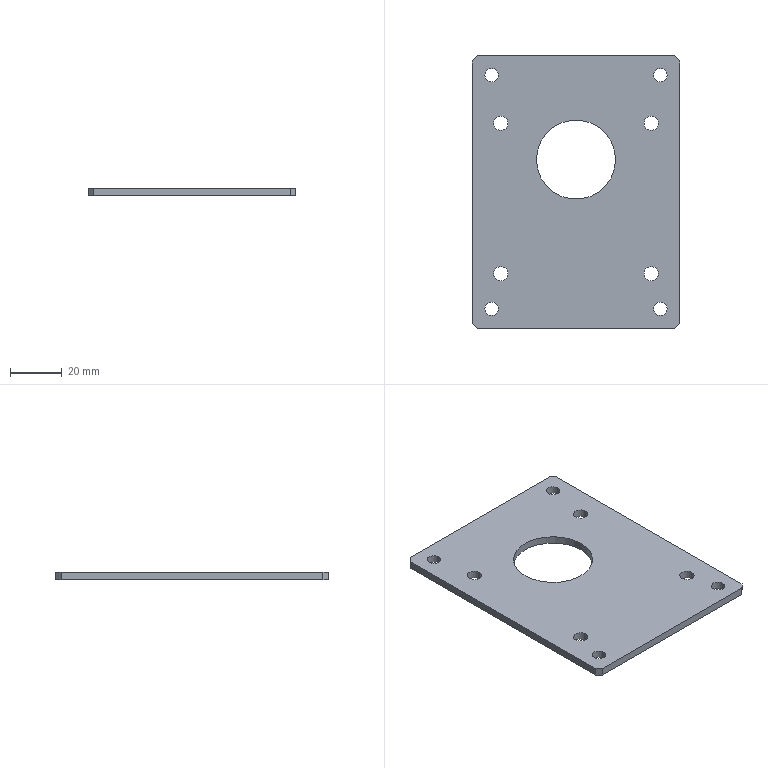Part | SolidWorks | features ICE 2, Chamfer 1, Extrusion 1, HoleWzd 1 | 1 solid | 28 faces | box 80 x 105 x 3 mm | volume 22444 mm3 | cylinder 18 | plane 10 | commonest cylinder face diameters 5.2 x8 5.5 x8 30.5 x2
STEP:
#1=CARTESIAN_POINT('',(13.759,21.009,3.));
#2=VERTEX_POINT('',#1);
#3=CARTESIAN_POINT('',(8.259,21.009,3.));
#4=VERTEX_POINT('',#3);
#5=CARTESIAN_POINT('',(11.009,21.009,3.));
#6=DIRECTION('',(0.,0.,-1.));
#7=DIRECTION('',(-1.,0.,0.));
#8=AXIS2_PLACEMENT_3D('',#5,#6,#7);
#9=CIRCLE('',#8,2.75);
#10=EDGE_CURVE('',#2,#4,#9,.T.);
#11=ORIENTED_EDGE('',*,*,#10,.F.);
#12=CARTESIAN_POINT('',(13.759,21.009,0.));
#13=VERTEX_POINT('',#12);
#14=CARTESIAN_POINT('',(13.759,21.009,3.));
#15=DIRECTION('',(0.,0.,-1.));
#16=VECTOR('',#15,1000.);
#17=LINE('',#14,#16);
#18=EDGE_CURVE('',#2,#13,#17,.T.);
#19=ORIENTED_EDGE('',*,*,#18,.T.);
#20=CARTESIAN_POINT('',(8.259,21.009,0.));
#21=VERTEX_POINT('',#20);
#22=CARTESIAN_POINT('',(11.009,21.009,0.));
#23=DIRECTION('',(0.,0.,-1.));
#24=DIRECTION('',(-1.,0.,0.));
#25=AXIS2_PLACEMENT_3D('',#22,#23,#24);
#26=CIRCLE('',#25,2.75);
#27=EDGE_CURVE('',#13,#21,#26,.T.);
#28=ORIENTED_EDGE('',*,*,#27,.T.);
#29=CARTESIAN_POINT('',(8.259,21.009,3.));
#30=DIRECTION('',(0.,0.,-1.));
#31=VECTOR('',#30,1000.);
#32=LINE('',#29,#31);
#33=EDGE_CURVE('',#4,#21,#32,.T.);
#34=ORIENTED_EDGE('',*,*,#33,.F.);
#35=EDGE_LOOP('',(#11,#19,#28,#34));
#36=FACE_OUTER_BOUND('',#35,.T.);
#37=CARTESIAN_POINT('',(11.009,21.009,3.));
#38=DIRECTION('',(0.,0.,-1.));
#39=DIRECTION('',(-1.,0.,0.));
#40=AXIS2_PLACEMENT_3D('',#37,#38,#39);
#41=CYLINDRICAL_SURFACE('',#40,2.75);
#42=ADVANCED_FACE('',(#36),#41,.F.);
#43=CARTESIAN_POINT('',(71.741,21.009,3.));
#44=VERTEX_POINT('',#43);
#45=CARTESIAN_POINT('',(66.241,21.009,3.));
#46=VERTEX_POINT('',#45);
#47=CARTESIAN_POINT('',(68.991,21.009,3.));
#48=DIRECTION('',(0.,0.,-1.));
#49=DIRECTION('',(-1.,0.,0.));
#50=AXIS2_PLACEMENT_3D('',#47,#48,#49);
#51=CIRCLE('',#50,2.75);
#52=EDGE_CURVE('',#44,#46,#51,.T.);
#53=ORIENTED_EDGE('',*,*,#52,.F.);
#54=CARTESIAN_POINT('',(71.741,21.009,0.));
#55=VERTEX_POINT('',#54);
#56=CARTESIAN_POINT('',(71.741,21.009,3.));
#57=DIRECTION('',(0.,0.,-1.));
#58=VECTOR('',#57,1000.);
#59=LINE('',#56,#58);
#60=EDGE_CURVE('',#44,#55,#59,.T.);
#61=ORIENTED_EDGE('',*,*,#60,.T.);
#62=CARTESIAN_POINT('',(66.241,21.009,0.));
#63=VERTEX_POINT('',#62);
#64=CARTESIAN_POINT('',(68.991,21.009,0.));
#65=DIRECTION('',(0.,0.,-1.));
#66=DIRECTION('',(-1.,0.,0.));
#67=AXIS2_PLACEMENT_3D('',#64,#65,#66);
#68=CIRCLE('',#67,2.75);
#69=EDGE_CURVE('',#55,#63,#68,.T.);
#70=ORIENTED_EDGE('',*,*,#69,.T.);
#71=CARTESIAN_POINT('',(66.241,21.009,3.));
#72=DIRECTION('',(0.,0.,-1.));
#73=VECTOR('',#72,1000.);
#74=LINE('',#71,#73);
#75=EDGE_CURVE('',#46,#63,#74,.T.);
#76=ORIENTED_EDGE('',*,*,#75,.F.);
#77=EDGE_LOOP('',(#53,#61,#70,#76));
#78=FACE_OUTER_BOUND('',#77,.T.);
#79=CARTESIAN_POINT('',(68.991,21.009,3.));
#80=DIRECTION('',(0.,0.,-1.));
#81=DIRECTION('',(-1.,0.,0.));
#82=AXIS2_PLACEMENT_3D('',#79,#80,#81);
#83=CYLINDRICAL_SURFACE('',#82,2.75);
#84=ADVANCED_FACE('',(#78),#83,.F.);
#85=CARTESIAN_POINT('',(13.759,78.991,3.));
#86=VERTEX_POINT('',#85);
#87=CARTESIAN_POINT('',(8.259,78.991,3.));
#88=VERTEX_POINT('',#87);
#89=CARTESIAN_POINT('',(11.009,78.991,3.));
#90=DIRECTION('',(0.,0.,-1.));
#91=DIRECTION('',(-1.,0.,0.));
#92=AXIS2_PLACEMENT_3D('',#89,#90,#91);
#93=CIRCLE('',#92,2.75);
#94=EDGE_CURVE('',#86,#88,#93,.T.);
#95=ORIENTED_EDGE('',*,*,#94,.F.);
#96=CARTESIAN_POINT('',(13.759,78.991,0.));
#97=VERTEX_POINT('',#96);
#98=CARTESIAN_POINT('',(13.759,78.991,3.));
#99=DIRECTION('',(0.,0.,-1.));
#100=VECTOR('',#99,1000.);
#101=LINE('',#98,#100);
#102=EDGE_CURVE('',#86,#97,#101,.T.);
#103=ORIENTED_EDGE('',*,*,#102,.T.);
#104=CARTESIAN_POINT('',(8.259,78.991,0.));
#105=VERTEX_POINT('',#104);
#106=CARTESIAN_POINT('',(11.009,78.991,0.));
#107=DIRECTION('',(0.,0.,-1.));
#108=DIRECTION('',(-1.,0.,0.));
#109=AXIS2_PLACEMENT_3D('',#106,#107,#108);
#110=CIRCLE('',#109,2.75);
#111=EDGE_CURVE('',#97,#105,#110,.T.);
#112=ORIENTED_EDGE('',*,*,#111,.T.);
#113=CARTESIAN_POINT('',(8.259,78.991,3.));
#114=DIRECTION('',(0.,0.,-1.));
#115=VECTOR('',#114,1000.);
#116=LINE('',#113,#115);
#117=EDGE_CURVE('',#88,#105,#116,.T.);
#118=ORIENTED_EDGE('',*,*,#117,.F.);
#119=EDGE_LOOP('',(#95,#103,#112,#118));
#120=FACE_OUTER_BOUND('',#119,.T.);
#121=CARTESIAN_POINT('',(11.009,78.991,3.));
#122=DIRECTION('',(0.,0.,-1.));
#123=DIRECTION('',(-1.,0.,0.));
#124=AXIS2_PLACEMENT_3D('',#121,#122,#123);
#125=CYLINDRICAL_SURFACE('',#124,2.75);
#126=ADVANCED_FACE('',(#120),#125,.F.);
#127=CARTESIAN_POINT('',(71.741,78.991,3.));
#128=VERTEX_POINT('',#127);
#129=CARTESIAN_POINT('',(66.241,78.991,3.));
#130=VERTEX_POINT('',#129);
#131=CARTESIAN_POINT('',(68.991,78.991,3.));
#132=DIRECTION('',(0.,0.,-1.));
#133=DIRECTION('',(-1.,0.,0.));
#134=AXIS2_PLACEMENT_3D('',#131,#132,#133);
#135=CIRCLE('',#134,2.75);
#136=EDGE_CURVE('',#128,#130,#135,.T.);
#137=ORIENTED_EDGE('',*,*,#136,.F.);
#138=CARTESIAN_POINT('',(71.741,78.991,0.));
#139=VERTEX_POINT('',#138);
#140=CARTESIAN_POINT('',(71.741,78.991,3.));
#141=DIRECTION('',(0.,0.,-1.));
#142=VECTOR('',#141,1000.);
#143=LINE('',#140,#142);
#144=EDGE_CURVE('',#128,#139,#143,.T.);
#145=ORIENTED_EDGE('',*,*,#144,.T.);
#146=CARTESIAN_POINT('',(66.241,78.991,0.));
#147=VERTEX_POINT('',#146);
#148=CARTESIAN_POINT('',(68.991,78.991,0.));
#149=DIRECTION('',(0.,0.,-1.));
#150=DIRECTION('',(-1.,0.,0.));
#151=AXIS2_PLACEMENT_3D('',#148,#149,#150);
#152=CIRCLE('',#151,2.75);
#153=EDGE_CURVE('',#139,#147,#152,.T.);
#154=ORIENTED_EDGE('',*,*,#153,.T.);
#155=CARTESIAN_POINT('',(66.241,78.991,3.));
#156=DIRECTION('',(0.,0.,-1.));
#157=VECTOR('',#156,1000.);
#158=LINE('',#155,#157);
#159=EDGE_CURVE('',#130,#147,#158,.T.);
#160=ORIENTED_EDGE('',*,*,#159,.F.);
#161=EDGE_LOOP('',(#137,#145,#154,#160));
#162=FACE_OUTER_BOUND('',#161,.T.);
#163=CARTESIAN_POINT('',(68.991,78.991,3.));
#164=DIRECTION('',(0.,0.,-1.));
#165=DIRECTION('',(-1.,0.,0.));
#166=AXIS2_PLACEMENT_3D('',#163,#164,#165);
#167=CYLINDRICAL_SURFACE('',#166,2.75);
#168=ADVANCED_FACE('',(#162),#167,.F.);
#169=CARTESIAN_POINT('',(55.25,65.,0.));
#170=VERTEX_POINT('',#169);
#171=CARTESIAN_POINT('',(24.75,65.,0.));
#172=VERTEX_POINT('',#171);
#173=CARTESIAN_POINT('',(40.,65.,0.));
#174=DIRECTION('',(0.,0.,-1.));
#175=DIRECTION('',(-1.,0.,0.));
#176=AXIS2_PLACEMENT_3D('',#173,#174,#175);
#177=CIRCLE('',#176,15.25);
#178=EDGE_CURVE('',#170,#172,#177,.T.);
#179=ORIENTED_EDGE('',*,*,#178,.T.);
#180=CARTESIAN_POINT('',(24.75,65.,3.));
#181=VERTEX_POINT('',#180);
#182=CARTESIAN_POINT('',(24.75,65.,-7.));
#183=DIRECTION('',(0.,0.,1.));
#184=VECTOR('',#183,1000.);
#185=LINE('',#182,#184);
#186=EDGE_CURVE('',#172,#181,#185,.T.);
#187=ORIENTED_EDGE('',*,*,#186,.T.);
#188=CARTESIAN_POINT('',(55.25,65.,3.));
#189=VERTEX_POINT('',#188);
#190=CARTESIAN_POINT('',(40.,65.,3.));
#191=DIRECTION('',(0.,0.,1.));
#192=DIRECTION('',(1.,0.,0.));
#193=AXIS2_PLACEMENT_3D('',#190,#191,#192);
#194=CIRCLE('',#193,15.25);
#195=EDGE_CURVE('',#181,#189,#194,.T.);
#196=ORIENTED_EDGE('',*,*,#195,.T.);
#197=CARTESIAN_POINT('',(55.25,65.,-7.));
#198=DIRECTION('',(0.,0.,1.));
#199=VECTOR('',#198,1000.);
#200=LINE('',#197,#199);
#201=EDGE_CURVE('',#170,#189,#200,.T.);
#202=ORIENTED_EDGE('',*,*,#201,.F.);
#203=EDGE_LOOP('',(#179,#187,#196,#202));
#204=FACE_OUTER_BOUND('',#203,.T.);
#205=CARTESIAN_POINT('',(40.,65.,-7.));
#206=DIRECTION('',(0.,0.,1.));
#207=DIRECTION('',(1.,0.,0.));
#208=AXIS2_PLACEMENT_3D('',#205,#206,#207);
#209=CYLINDRICAL_SURFACE('',#208,15.25);
#210=ADVANCED_FACE('',(#204),#209,.F.);
#211=CARTESIAN_POINT('',(75.1,7.5,0.));
#212=VERTEX_POINT('',#211);
#213=CARTESIAN_POINT('',(69.9,7.5,0.));
#214=VERTEX_POINT('',#213);
#215=CARTESIAN_POINT('',(72.5,7.5,0.));
#216=DIRECTION('',(0.,0.,-1.));
#217=DIRECTION('',(-1.,0.,0.));
#218=AXIS2_PLACEMENT_3D('',#215,#216,#217);
#219=CIRCLE('',#218,2.6);
#220=EDGE_CURVE('',#212,#214,#219,.T.);
#221=ORIENTED_EDGE('',*,*,#220,.T.);
#222=CARTESIAN_POINT('',(69.9,7.5,3.));
#223=VERTEX_POINT('',#222);
#224=CARTESIAN_POINT('',(69.9,7.5,-7.));
#225=DIRECTION('',(0.,0.,1.));
#226=VECTOR('',#225,1000.);
#227=LINE('',#224,#226);
#228=EDGE_CURVE('',#214,#223,#227,.T.);
#229=ORIENTED_EDGE('',*,*,#228,.T.);
#230=CARTESIAN_POINT('',(75.1,7.5,3.));
#231=VERTEX_POINT('',#230);
#232=CARTESIAN_POINT('',(72.5,7.5,3.));
#233=DIRECTION('',(0.,0.,1.));
#234=DIRECTION('',(1.,0.,0.));
#235=AXIS2_PLACEMENT_3D('',#232,#233,#234);
#236=CIRCLE('',#235,2.6);
#237=EDGE_CURVE('',#223,#231,#236,.T.);
#238=ORIENTED_EDGE('',*,*,#237,.T.);
#239=CARTESIAN_POINT('',(75.1,7.5,-7.));
#240=DIRECTION('',(0.,0.,1.));
#241=VECTOR('',#240,1000.);
#242=LINE('',#239,#241);
#243=EDGE_CURVE('',#212,#231,#242,.T.);
#244=ORIENTED_EDGE('',*,*,#243,.F.);
#245=EDGE_LOOP('',(#221,#229,#238,#244));
#246=FACE_OUTER_BOUND('',#245,.T.);
#247=CARTESIAN_POINT('',(72.5,7.5,-7.));
#248=DIRECTION('',(0.,0.,1.));
#249=DIRECTION('',(1.,0.,0.));
#250=AXIS2_PLACEMENT_3D('',#247,#248,#249);
#251=CYLINDRICAL_SURFACE('',#250,2.6);
#252=ADVANCED_FACE('',(#246),#251,.F.);
#253=CARTESIAN_POINT('',(10.1,7.5,0.));
#254=VERTEX_POINT('',#253);
#255=CARTESIAN_POINT('',(4.9,7.5,0.));
#256=VERTEX_POINT('',#255);
#257=CARTESIAN_POINT('',(7.5,7.5,0.));
#258=DIRECTION('',(0.,0.,-1.));
#259=DIRECTION('',(-1.,0.,0.));
#260=AXIS2_PLACEMENT_3D('',#257,#258,#259);
#261=CIRCLE('',#260,2.6);
#262=EDGE_CURVE('',#254,#256,#261,.T.);
#263=ORIENTED_EDGE('',*,*,#262,.T.);
#264=CARTESIAN_POINT('',(4.9,7.5,3.));
#265=VERTEX_POINT('',#264);
#266=CARTESIAN_POINT('',(4.9,7.5,-7.));
#267=DIRECTION('',(0.,0.,1.));
#268=VECTOR('',#267,1000.);
#269=LINE('',#266,#268);
#270=EDGE_CURVE('',#256,#265,#269,.T.);
#271=ORIENTED_EDGE('',*,*,#270,.T.);
#272=CARTESIAN_POINT('',(10.1,7.5,3.));
#273=VERTEX_POINT('',#272);
#274=CARTESIAN_POINT('',(7.5,7.5,3.));
#275=DIRECTION('',(0.,0.,1.));
#276=DIRECTION('',(1.,0.,0.));
#277=AXIS2_PLACEMENT_3D('',#274,#275,#276);
#278=CIRCLE('',#277,2.6);
#279=EDGE_CURVE('',#265,#273,#278,.T.);
#280=ORIENTED_EDGE('',*,*,#279,.T.);
#281=CARTESIAN_POINT('',(10.1,7.5,-7.));
#282=DIRECTION('',(0.,0.,1.));
#283=VECTOR('',#282,1000.);
#284=LINE('',#281,#283);
#285=EDGE_CURVE('',#254,#273,#284,.T.);
#286=ORIENTED_EDGE('',*,*,#285,.F.);
#287=EDGE_LOOP('',(#263,#271,#280,#286));
#288=FACE_OUTER_BOUND('',#287,.T.);
#289=CARTESIAN_POINT('',(7.5,7.5,-7.));
#290=DIRECTION('',(0.,0.,1.));
#291=DIRECTION('',(1.,0.,0.));
#292=AXIS2_PLACEMENT_3D('',#289,#290,#291);
#293=CYLINDRICAL_SURFACE('',#292,2.6);
#294=ADVANCED_FACE('',(#288),#293,.F.);
#295=CARTESIAN_POINT('',(75.1,97.5,0.));
#296=VERTEX_POINT('',#295);
#297=CARTESIAN_POINT('',(69.9,97.5,0.));
#298=VERTEX_POINT('',#297);
#299=CARTESIAN_POINT('',(72.5,97.5,0.));
#300=DIRECTION('',(0.,0.,-1.));
#301=DIRECTION('',(-1.,0.,0.));
#302=AXIS2_PLACEMENT_3D('',#299,#300,#301);
#303=CIRCLE('',#302,2.6);
#304=EDGE_CURVE('',#296,#298,#303,.T.);
#305=ORIENTED_EDGE('',*,*,#304,.T.);
#306=CARTESIAN_POINT('',(69.9,97.5,3.));
#307=VERTEX_POINT('',#306);
#308=CARTESIAN_POINT('',(69.9,97.5,-7.));
#309=DIRECTION('',(0.,0.,1.));
#310=VECTOR('',#309,1000.);
#311=LINE('',#308,#310);
#312=EDGE_CURVE('',#298,#307,#311,.T.);
#313=ORIENTED_EDGE('',*,*,#312,.T.);
#314=CARTESIAN_POINT('',(75.1,97.5,3.));
#315=VERTEX_POINT('',#314);
#316=CARTESIAN_POINT('',(72.5,97.5,3.));
#317=DIRECTION('',(0.,0.,1.));
#318=DIRECTION('',(1.,0.,0.));
#319=AXIS2_PLACEMENT_3D('',#316,#317,#318);
#320=CIRCLE('',#319,2.6);
#321=EDGE_CURVE('',#307,#315,#320,.T.);
#322=ORIENTED_EDGE('',*,*,#321,.T.);
#323=CARTESIAN_POINT('',(75.1,97.5,-7.));
#324=DIRECTION('',(0.,0.,1.));
#325=VECTOR('',#324,1000.);
#326=LINE('',#323,#325);
#327=EDGE_CURVE('',#296,#315,#326,.T.);
#328=ORIENTED_EDGE('',*,*,#327,.F.);
#329=EDGE_LOOP('',(#305,#313,#322,#328));
#330=FACE_OUTER_BOUND('',#329,.T.);
#331=CARTESIAN_POINT('',(72.5,97.5,-7.));
#332=DIRECTION('',(0.,0.,1.));
#333=DIRECTION('',(1.,0.,0.));
#334=AXIS2_PLACEMENT_3D('',#331,#332,#333);
#335=CYLINDRICAL_SURFACE('',#334,2.6);
#336=ADVANCED_FACE('',(#330),#335,.F.);
#337=CARTESIAN_POINT('',(10.1,97.5,0.));
#338=VERTEX_POINT('',#337);
#339=CARTESIAN_POINT('',(4.9,97.5,0.));
#340=VERTEX_POINT('',#339);
#341=CARTESIAN_POINT('',(7.5,97.5,0.));
#342=DIRECTION('',(0.,0.,-1.));
#343=DIRECTION('',(-1.,0.,0.));
#344=AXIS2_PLACEMENT_3D('',#341,#342,#343);
#345=CIRCLE('',#344,2.6);
#346=EDGE_CURVE('',#338,#340,#345,.T.);
#347=ORIENTED_EDGE('',*,*,#346,.T.);
#348=CARTESIAN_POINT('',(4.9,97.5,3.));
#349=VERTEX_POINT('',#348);
#350=CARTESIAN_POINT('',(4.9,97.5,-7.));
#351=DIRECTION('',(0.,0.,1.));
#352=VECTOR('',#351,1000.);
#353=LINE('',#350,#352);
#354=EDGE_CURVE('',#340,#349,#353,.T.);
#355=ORIENTED_EDGE('',*,*,#354,.T.);
#356=CARTESIAN_POINT('',(10.1,97.5,3.));
#357=VERTEX_POINT('',#356);
#358=CARTESIAN_POINT('',(7.5,97.5,3.));
#359=DIRECTION('',(0.,0.,1.));
#360=DIRECTION('',(1.,0.,0.));
#361=AXIS2_PLACEMENT_3D('',#358,#359,#360);
#362=CIRCLE('',#361,2.6);
#363=EDGE_CURVE('',#349,#357,#362,.T.);
#364=ORIENTED_EDGE('',*,*,#363,.T.);
#365=CARTESIAN_POINT('',(10.1,97.5,-7.));
#366=DIRECTION('',(0.,0.,1.));
#367=VECTOR('',#366,1000.);
#368=LINE('',#365,#367);
#369=EDGE_CURVE('',#338,#357,#368,.T.);
#370=ORIENTED_EDGE('',*,*,#369,.F.);
#371=EDGE_LOOP('',(#347,#355,#364,#370));
#372=FACE_OUTER_BOUND('',#371,.T.);
#373=CARTESIAN_POINT('',(7.5,97.5,-7.));
#374=DIRECTION('',(0.,0.,1.));
#375=DIRECTION('',(1.,0.,0.));
#376=AXIS2_PLACEMENT_3D('',#373,#374,#375);
#377=CYLINDRICAL_SURFACE('',#376,2.6);
#378=ADVANCED_FACE('',(#372),#377,.F.);
#379=CARTESIAN_POINT('',(0.,103.,0.));
#380=VERTEX_POINT('',#379);
#381=CARTESIAN_POINT('',(0.,2.,0.));
#382=VERTEX_POINT('',#381);
#383=CARTESIAN_POINT('',(0.,0.,0.));
#384=DIRECTION('',(0.,-1.,0.));
#385=VECTOR('',#384,1000.);
#386=LINE('',#383,#385);
#387=EDGE_CURVE('',#380,#382,#386,.T.);
#388=ORIENTED_EDGE('',*,*,#387,.T.);
#389=CARTESIAN_POINT('',(0.,2.,3.));
#390=VERTEX_POINT('',#389);
#391=CARTESIAN_POINT('',(0.,2.,3.));
#392=DIRECTION('',(0.,0.,1.));
#393=VECTOR('',#392,1000.);
#394=LINE('',#391,#393);
#395=EDGE_CURVE('',#382,#390,#394,.T.);
#396=ORIENTED_EDGE('',*,*,#395,.T.);
#397=CARTESIAN_POINT('',(0.,103.,3.));
#398=VERTEX_POINT('',#397);
#399=CARTESIAN_POINT('',(0.,0.,3.));
#400=DIRECTION('',(0.,-1.,0.));
#401=VECTOR('',#400,1000.);
#402=LINE('',#399,#401);
#403=EDGE_CURVE('',#398,#390,#402,.T.);
#404=ORIENTED_EDGE('',*,*,#403,.F.);
#405=CARTESIAN_POINT('',(0.,103.,3.));
#406=DIRECTION('',(0.,0.,-1.));
#407=VECTOR('',#406,1000.);
#408=LINE('',#405,#407);
#409=EDGE_CURVE('',#398,#380,#408,.T.);
#410=ORIENTED_EDGE('',*,*,#409,.T.);
#411=EDGE_LOOP('',(#388,#396,#404,#410));
#412=FACE_OUTER_BOUND('',#411,.T.);
#413=CARTESIAN_POINT('',(0.,0.,3.));
#414=DIRECTION('',(1.,0.,0.));
#415=DIRECTION('',(0.,0.,-1.));
#416=AXIS2_PLACEMENT_3D('',#413,#414,#415);
#417=PLANE('',#416);
#418=ADVANCED_FACE('',(#412),#417,.F.);
#419=CARTESIAN_POINT('',(2.,0.,3.));
#420=VERTEX_POINT('',#419);
#421=CARTESIAN_POINT('',(78.,0.,3.));
#422=VERTEX_POINT('',#421);
#423=CARTESIAN_POINT('',(0.,0.,3.));
#424=DIRECTION('',(1.,0.,0.));
#425=VECTOR('',#424,1000.);
#426=LINE('',#423,#425);
#427=EDGE_CURVE('',#420,#422,#426,.T.);
#428=ORIENTED_EDGE('',*,*,#427,.F.);
#429=CARTESIAN_POINT('',(2.,0.,0.));
#430=VERTEX_POINT('',#429);
#431=CARTESIAN_POINT('',(2.,0.,3.));
#432=DIRECTION('',(0.,0.,-1.));
#433=VECTOR('',#432,1000.);
#434=LINE('',#431,#433);
#435=EDGE_CURVE('',#420,#430,#434,.T.);
#436=ORIENTED_EDGE('',*,*,#435,.T.);
#437=CARTESIAN_POINT('',(78.,0.,0.));
#438=VERTEX_POINT('',#437);
#439=CARTESIAN_POINT('',(0.,0.,0.));
#440=DIRECTION('',(1.,0.,0.));
#441=VECTOR('',#440,1000.);
#442=LINE('',#439,#441);
#443=EDGE_CURVE('',#430,#438,#442,.T.);
#444=ORIENTED_EDGE('',*,*,#443,.T.);
#445=CARTESIAN_POINT('',(78.,0.,3.));
#446=DIRECTION('',(0.,0.,1.));
#447=VECTOR('',#446,1000.);
#448=LINE('',#445,#447);
#449=EDGE_CURVE('',#438,#422,#448,.T.);
#450=ORIENTED_EDGE('',*,*,#449,.T.);
#451=EDGE_LOOP('',(#428,#436,#444,#450));
#452=FACE_OUTER_BOUND('',#451,.T.);
#453=CARTESIAN_POINT('',(0.,0.,3.));
#454=DIRECTION('',(0.,1.,0.));
#455=DIRECTION('',(0.,0.,1.));
#456=AXIS2_PLACEMENT_3D('',#453,#454,#455);
#457=PLANE('',#456);
#458=ADVANCED_FACE('',(#452),#457,.F.);
#459=CARTESIAN_POINT('',(80.,2.,3.));
#460=VERTEX_POINT('',#459);
#461=CARTESIAN_POINT('',(80.,103.,3.));
#462=VERTEX_POINT('',#461);
#463=CARTESIAN_POINT('',(80.,0.,3.));
#464=DIRECTION('',(0.,1.,0.));
#465=VECTOR('',#464,1000.);
#466=LINE('',#463,#465);
#467=EDGE_CURVE('',#460,#462,#466,.T.);
#468=ORIENTED_EDGE('',*,*,#467,.F.);
#469=CARTESIAN_POINT('',(80.,2.,0.));
#470=VERTEX_POINT('',#469);
#471=CARTESIAN_POINT('',(80.,2.,3.));
#472=DIRECTION('',(0.,0.,-1.));
#473=VECTOR('',#472,1000.);
#474=LINE('',#471,#473);
#475=EDGE_CURVE('',#460,#470,#474,.T.);
#476=ORIENTED_EDGE('',*,*,#475,.T.);
#477=CARTESIAN_POINT('',(80.,103.,0.));
#478=VERTEX_POINT('',#477);
#479=CARTESIAN_POINT('',(80.,0.,0.));
#480=DIRECTION('',(0.,1.,0.));
#481=VECTOR('',#480,1000.);
#482=LINE('',#479,#481);
#483=EDGE_CURVE('',#470,#478,#482,.T.);
#484=ORIENTED_EDGE('',*,*,#483,.T.);
#485=CARTESIAN_POINT('',(80.,103.,3.));
#486=DIRECTION('',(0.,0.,1.));
#487=VECTOR('',#486,1000.);
#488=LINE('',#485,#487);
#489=EDGE_CURVE('',#478,#462,#488,.T.);
#490=ORIENTED_EDGE('',*,*,#489,.T.);
#491=EDGE_LOOP('',(#468,#476,#484,#490));
#492=FACE_OUTER_BOUND('',#491,.T.);
#493=CARTESIAN_POINT('',(80.,0.,3.));
#494=DIRECTION('',(-1.,0.,0.));
#495=DIRECTION('',(0.,0.,1.));
#496=AXIS2_PLACEMENT_3D('',#493,#494,#495);
#497=PLANE('',#496);
#498=ADVANCED_FACE('',(#492),#497,.F.);
#499=CARTESIAN_POINT('',(78.,105.,0.));
#500=VERTEX_POINT('',#499);
#501=CARTESIAN_POINT('',(2.,105.,0.));
#502=VERTEX_POINT('',#501);
#503=CARTESIAN_POINT('',(0.,105.,0.));
#504=DIRECTION('',(-1.,0.,0.));
#505=VECTOR('',#504,1000.);
#506=LINE('',#503,#505);
#507=EDGE_CURVE('',#500,#502,#506,.T.);
#508=ORIENTED_EDGE('',*,*,#507,.T.);
#509=CARTESIAN_POINT('',(2.,105.,3.));
#510=VERTEX_POINT('',#509);
#511=CARTESIAN_POINT('',(2.,105.,3.));
#512=DIRECTION('',(0.,0.,1.));
#513=VECTOR('',#512,1000.);
#514=LINE('',#511,#513);
#515=EDGE_CURVE('',#502,#510,#514,.T.);
#516=ORIENTED_EDGE('',*,*,#515,.T.);
#517=CARTESIAN_POINT('',(78.,105.,3.));
#518=VERTEX_POINT('',#517);
#519=CARTESIAN_POINT('',(0.,105.,3.));
#520=DIRECTION('',(-1.,0.,0.));
#521=VECTOR('',#520,1000.);
#522=LINE('',#519,#521);
#523=EDGE_CURVE('',#518,#510,#522,.T.);
#524=ORIENTED_EDGE('',*,*,#523,.F.);
#525=CARTESIAN_POINT('',(78.,105.,3.));
#526=DIRECTION('',(0.,0.,-1.));
#527=VECTOR('',#526,1000.);
#528=LINE('',#525,#527);
#529=EDGE_CURVE('',#518,#500,#528,.T.);
#530=ORIENTED_EDGE('',*,*,#529,.T.);
#531=EDGE_LOOP('',(#508,#516,#524,#530));
#532=FACE_OUTER_BOUND('',#531,.T.);
#533=CARTESIAN_POINT('',(0.,105.,3.));
#534=DIRECTION('',(0.,-1.,0.));
#535=DIRECTION('',(0.,0.,-1.));
#536=AXIS2_PLACEMENT_3D('',#533,#534,#535);
#537=PLANE('',#536);
#538=ADVANCED_FACE('',(#532),#537,.F.);
#539=CARTESIAN_POINT('',(11.009,21.009,3.));
#540=DIRECTION('',(0.,0.,-1.));
#541=DIRECTION('',(-1.,0.,0.));
#542=AXIS2_PLACEMENT_3D('',#539,#540,#541);
#543=CIRCLE('',#542,2.75);
#544=EDGE_CURVE('',#4,#2,#543,.T.);
#545=ORIENTED_EDGE('',*,*,#544,.T.);
#546=ORIENTED_EDGE('',*,*,#10,.T.);
#547=EDGE_LOOP('',(#545,#546));
#548=FACE_BOUND('',#547,.T.);
#549=CARTESIAN_POINT('',(68.991,21.009,3.));
#550=DIRECTION('',(0.,0.,-1.));
#551=DIRECTION('',(-1.,0.,0.));
#552=AXIS2_PLACEMENT_3D('',#549,#550,#551);
#553=CIRCLE('',#552,2.75);
#554=EDGE_CURVE('',#46,#44,#553,.T.);
#555=ORIENTED_EDGE('',*,*,#554,.T.);
#556=ORIENTED_EDGE('',*,*,#52,.T.);
#557=EDGE_LOOP('',(#555,#556));
#558=FACE_BOUND('',#557,.T.);
#559=CARTESIAN_POINT('',(11.009,78.991,3.));
#560=DIRECTION('',(0.,0.,-1.));
#561=DIRECTION('',(-1.,0.,0.));
#562=AXIS2_PLACEMENT_3D('',#559,#560,#561);
#563=CIRCLE('',#562,2.75);
#564=EDGE_CURVE('',#88,#86,#563,.T.);
#565=ORIENTED_EDGE('',*,*,#564,.T.);
#566=ORIENTED_EDGE('',*,*,#94,.T.);
#567=EDGE_LOOP('',(#565,#566));
#568=FACE_BOUND('',#567,.T.);
#569=CARTESIAN_POINT('',(68.991,78.991,3.));
#570=DIRECTION('',(0.,0.,-1.));
#571=DIRECTION('',(-1.,0.,0.));
#572=AXIS2_PLACEMENT_3D('',#569,#570,#571);
#573=CIRCLE('',#572,2.75);
#574=EDGE_CURVE('',#130,#128,#573,.T.);
#575=ORIENTED_EDGE('',*,*,#574,.T.);
#576=ORIENTED_EDGE('',*,*,#136,.T.);
#577=EDGE_LOOP('',(#575,#576));
#578=FACE_BOUND('',#577,.T.);
#579=CARTESIAN_POINT('',(40.,65.,3.));
#580=DIRECTION('',(0.,0.,1.));
#581=DIRECTION('',(1.,0.,0.));
#582=AXIS2_PLACEMENT_3D('',#579,#580,#581);
#583=CIRCLE('',#582,15.25);
#584=EDGE_CURVE('',#189,#181,#583,.T.);
#585=ORIENTED_EDGE('',*,*,#584,.F.);
#586=ORIENTED_EDGE('',*,*,#195,.F.);
#587=EDGE_LOOP('',(#585,#586));
#588=FACE_BOUND('',#587,.T.);
#589=CARTESIAN_POINT('',(72.5,7.5,3.));
#590=DIRECTION('',(0.,0.,1.));
#591=DIRECTION('',(1.,0.,0.));
#592=AXIS2_PLACEMENT_3D('',#589,#590,#591);
#593=CIRCLE('',#592,2.6);
#594=EDGE_CURVE('',#231,#223,#593,.T.);
#595=ORIENTED_EDGE('',*,*,#594,.F.);
#596=ORIENTED_EDGE('',*,*,#237,.F.);
#597=EDGE_LOOP('',(#595,#596));
#598=FACE_BOUND('',#597,.T.);
#599=CARTESIAN_POINT('',(7.5,7.5,3.));
#600=DIRECTION('',(0.,0.,1.));
#601=DIRECTION('',(1.,0.,0.));
#602=AXIS2_PLACEMENT_3D('',#599,#600,#601);
#603=CIRCLE('',#602,2.6);
#604=EDGE_CURVE('',#273,#265,#603,.T.);
#605=ORIENTED_EDGE('',*,*,#604,.F.);
#606=ORIENTED_EDGE('',*,*,#279,.F.);
#607=EDGE_LOOP('',(#605,#606));
#608=FACE_BOUND('',#607,.T.);
#609=CARTESIAN_POINT('',(72.5,97.5,3.));
#610=DIRECTION('',(0.,0.,1.));
#611=DIRECTION('',(1.,0.,0.));
#612=AXIS2_PLACEMENT_3D('',#609,#610,#611);
#613=CIRCLE('',#612,2.6);
#614=EDGE_CURVE('',#315,#307,#613,.T.);
#615=ORIENTED_EDGE('',*,*,#614,.F.);
#616=ORIENTED_EDGE('',*,*,#321,.F.);
#617=EDGE_LOOP('',(#615,#616));
#618=FACE_BOUND('',#617,.T.);
#619=CARTESIAN_POINT('',(7.5,97.5,3.));
#620=DIRECTION('',(0.,0.,1.));
#621=DIRECTION('',(1.,0.,0.));
#622=AXIS2_PLACEMENT_3D('',#619,#620,#621);
#623=CIRCLE('',#622,2.6);
#624=EDGE_CURVE('',#357,#349,#623,.T.);
#625=ORIENTED_EDGE('',*,*,#624,.F.);
#626=ORIENTED_EDGE('',*,*,#363,.F.);
#627=EDGE_LOOP('',(#625,#626));
#628=FACE_BOUND('',#627,.T.);
#629=ORIENTED_EDGE('',*,*,#403,.T.);
#630=CARTESIAN_POINT('',(2.,0.,3.));
#631=DIRECTION('',(0.7071,-0.7071,0.));
#632=VECTOR('',#631,1000.);
#633=LINE('',#630,#632);
#634=EDGE_CURVE('',#390,#420,#633,.T.);
#635=ORIENTED_EDGE('',*,*,#634,.T.);
#636=ORIENTED_EDGE('',*,*,#427,.T.);
#637=CARTESIAN_POINT('',(80.,2.,3.));
#638=DIRECTION('',(0.7071,0.7071,0.));
#639=VECTOR('',#638,1000.);
#640=LINE('',#637,#639);
#641=EDGE_CURVE('',#422,#460,#640,.T.);
#642=ORIENTED_EDGE('',*,*,#641,.T.);
#643=ORIENTED_EDGE('',*,*,#467,.T.);
#644=CARTESIAN_POINT('',(78.,105.,3.));
#645=DIRECTION('',(-0.7071,0.7071,0.));
#646=VECTOR('',#645,1000.);
#647=LINE('',#644,#646);
#648=EDGE_CURVE('',#462,#518,#647,.T.);
#649=ORIENTED_EDGE('',*,*,#648,.T.);
#650=ORIENTED_EDGE('',*,*,#523,.T.);
#651=CARTESIAN_POINT('',(0.,103.,3.));
#652=DIRECTION('',(-0.7071,-0.7071,0.));
#653=VECTOR('',#652,1000.);
#654=LINE('',#651,#653);
#655=EDGE_CURVE('',#510,#398,#654,.T.);
#656=ORIENTED_EDGE('',*,*,#655,.T.);
#657=EDGE_LOOP('',(#629,#635,#636,#642,#643,#649,#650,#656));
#658=FACE_OUTER_BOUND('',#657,.T.);
#659=CARTESIAN_POINT('',(0.,105.,3.));
#660=DIRECTION('',(0.,0.,-1.));
#661=DIRECTION('',(-1.,0.,0.));
#662=AXIS2_PLACEMENT_3D('',#659,#660,#661);
#663=PLANE('',#662);
#664=ADVANCED_FACE('',(#548,#558,#568,#578,#588,#598,#608,#618,#628,#658),#663,.F.);
#665=CARTESIAN_POINT('',(11.009,21.009,0.));
#666=DIRECTION('',(0.,0.,-1.));
#667=DIRECTION('',(-1.,0.,0.));
#668=AXIS2_PLACEMENT_3D('',#665,#666,#667);
#669=CIRCLE('',#668,2.75);
#670=EDGE_CURVE('',#21,#13,#669,.T.);
#671=ORIENTED_EDGE('',*,*,#670,.F.);
#672=ORIENTED_EDGE('',*,*,#27,.F.);
#673=EDGE_LOOP('',(#671,#672));
#674=FACE_BOUND('',#673,.T.);
#675=CARTESIAN_POINT('',(68.991,21.009,0.));
#676=DIRECTION('',(0.,0.,-1.));
#677=DIRECTION('',(-1.,0.,0.));
#678=AXIS2_PLACEMENT_3D('',#675,#676,#677);
#679=CIRCLE('',#678,2.75);
#680=EDGE_CURVE('',#63,#55,#679,.T.);
#681=ORIENTED_EDGE('',*,*,#680,.F.);
#682=ORIENTED_EDGE('',*,*,#69,.F.);
#683=EDGE_LOOP('',(#681,#682));
#684=FACE_BOUND('',#683,.T.);
#685=CARTESIAN_POINT('',(11.009,78.991,0.));
#686=DIRECTION('',(0.,0.,-1.));
#687=DIRECTION('',(-1.,0.,0.));
#688=AXIS2_PLACEMENT_3D('',#685,#686,#687);
#689=CIRCLE('',#688,2.75);
#690=EDGE_CURVE('',#105,#97,#689,.T.);
#691=ORIENTED_EDGE('',*,*,#690,.F.);
#692=ORIENTED_EDGE('',*,*,#111,.F.);
#693=EDGE_LOOP('',(#691,#692));
#694=FACE_BOUND('',#693,.T.);
#695=CARTESIAN_POINT('',(68.991,78.991,0.));
#696=DIRECTION('',(0.,0.,-1.));
#697=DIRECTION('',(-1.,0.,0.));
#698=AXIS2_PLACEMENT_3D('',#695,#696,#697);
#699=CIRCLE('',#698,2.75);
#700=EDGE_CURVE('',#147,#139,#699,.T.);
#701=ORIENTED_EDGE('',*,*,#700,.F.);
#702=ORIENTED_EDGE('',*,*,#153,.F.);
#703=EDGE_LOOP('',(#701,#702));
#704=FACE_BOUND('',#703,.T.);
#705=ORIENTED_EDGE('',*,*,#178,.F.);
#706=CARTESIAN_POINT('',(40.,65.,0.));
#707=DIRECTION('',(0.,0.,-1.));
#708=DIRECTION('',(-1.,0.,0.));
#709=AXIS2_PLACEMENT_3D('',#706,#707,#708);
#710=CIRCLE('',#709,15.25);
#711=EDGE_CURVE('',#172,#170,#710,.T.);
#712=ORIENTED_EDGE('',*,*,#711,.F.);
#713=EDGE_LOOP('',(#705,#712));
#714=FACE_BOUND('',#713,.T.);
#715=ORIENTED_EDGE('',*,*,#220,.F.);
#716=CARTESIAN_POINT('',(72.5,7.5,0.));
#717=DIRECTION('',(0.,0.,-1.));
#718=DIRECTION('',(-1.,0.,0.));
#719=AXIS2_PLACEMENT_3D('',#716,#717,#718);
#720=CIRCLE('',#719,2.6);
#721=EDGE_CURVE('',#214,#212,#720,.T.);
#722=ORIENTED_EDGE('',*,*,#721,.F.);
#723=EDGE_LOOP('',(#715,#722));
#724=FACE_BOUND('',#723,.T.);
#725=ORIENTED_EDGE('',*,*,#262,.F.);
#726=CARTESIAN_POINT('',(7.5,7.5,0.));
#727=DIRECTION('',(0.,0.,-1.));
#728=DIRECTION('',(-1.,0.,0.));
#729=AXIS2_PLACEMENT_3D('',#726,#727,#728);
#730=CIRCLE('',#729,2.6);
#731=EDGE_CURVE('',#256,#254,#730,.T.);
#732=ORIENTED_EDGE('',*,*,#731,.F.);
#733=EDGE_LOOP('',(#725,#732));
#734=FACE_BOUND('',#733,.T.);
#735=ORIENTED_EDGE('',*,*,#304,.F.);
#736=CARTESIAN_POINT('',(72.5,97.5,0.));
#737=DIRECTION('',(0.,0.,-1.));
#738=DIRECTION('',(-1.,0.,0.));
#739=AXIS2_PLACEMENT_3D('',#736,#737,#738);
#740=CIRCLE('',#739,2.6);
#741=EDGE_CURVE('',#298,#296,#740,.T.);
#742=ORIENTED_EDGE('',*,*,#741,.F.);
#743=EDGE_LOOP('',(#735,#742));
#744=FACE_BOUND('',#743,.T.);
#745=ORIENTED_EDGE('',*,*,#346,.F.);
#746=CARTESIAN_POINT('',(7.5,97.5,0.));
#747=DIRECTION('',(0.,0.,-1.));
#748=DIRECTION('',(-1.,0.,0.));
#749=AXIS2_PLACEMENT_3D('',#746,#747,#748);
#750=CIRCLE('',#749,2.6);
#751=EDGE_CURVE('',#340,#338,#750,.T.);
#752=ORIENTED_EDGE('',*,*,#751,.F.);
#753=EDGE_LOOP('',(#745,#752));
#754=FACE_BOUND('',#753,.T.);
#755=ORIENTED_EDGE('',*,*,#443,.F.);
#756=CARTESIAN_POINT('',(-51.5,53.5,0.));
#757=DIRECTION('',(-0.7071,0.7071,0.));
#758=VECTOR('',#757,1000.);
#759=LINE('',#756,#758);
#760=EDGE_CURVE('',#430,#382,#759,.T.);
#761=ORIENTED_EDGE('',*,*,#760,.T.);
#762=ORIENTED_EDGE('',*,*,#387,.F.);
#763=CARTESIAN_POINT('',(1.,104.,0.));
#764=DIRECTION('',(0.7071,0.7071,0.));
#765=VECTOR('',#764,1000.);
#766=LINE('',#763,#765);
#767=EDGE_CURVE('',#380,#502,#766,.T.);
#768=ORIENTED_EDGE('',*,*,#767,.T.);
#769=ORIENTED_EDGE('',*,*,#507,.F.);
#770=CARTESIAN_POINT('',(39.,144.,0.));
#771=DIRECTION('',(0.7071,-0.7071,0.));
#772=VECTOR('',#771,1000.);
#773=LINE('',#770,#772);
#774=EDGE_CURVE('',#500,#478,#773,.T.);
#775=ORIENTED_EDGE('',*,*,#774,.T.);
#776=ORIENTED_EDGE('',*,*,#483,.F.);
#777=CARTESIAN_POINT('',(91.5,13.5,0.));
#778=DIRECTION('',(-0.7071,-0.7071,0.));
#779=VECTOR('',#778,1000.);
#780=LINE('',#777,#779);
#781=EDGE_CURVE('',#470,#438,#780,.T.);
#782=ORIENTED_EDGE('',*,*,#781,.T.);
#783=EDGE_LOOP('',(#755,#761,#762,#768,#769,#775,#776,#782));
#784=FACE_OUTER_BOUND('',#783,.T.);
#785=CARTESIAN_POINT('',(0.,105.,0.));
#786=DIRECTION('',(0.,0.,-1.));
#787=DIRECTION('',(-1.,0.,0.));
#788=AXIS2_PLACEMENT_3D('',#785,#786,#787);
#789=PLANE('',#788);
#790=ADVANCED_FACE('',(#674,#684,#694,#704,#714,#724,#734,#744,#754,#784),#789,.T.);
#791=ORIENTED_EDGE('',*,*,#354,.F.);
#792=ORIENTED_EDGE('',*,*,#751,.T.);
#793=ORIENTED_EDGE('',*,*,#369,.T.);
#794=ORIENTED_EDGE('',*,*,#624,.T.);
#795=EDGE_LOOP('',(#791,#792,#793,#794));
#796=FACE_OUTER_BOUND('',#795,.T.);
#797=CARTESIAN_POINT('',(7.5,97.5,-7.));
#798=DIRECTION('',(0.,0.,1.));
#799=DIRECTION('',(1.,0.,0.));
#800=AXIS2_PLACEMENT_3D('',#797,#798,#799);
#801=CYLINDRICAL_SURFACE('',#800,2.6);
#802=ADVANCED_FACE('',(#796),#801,.F.);
#803=ORIENTED_EDGE('',*,*,#312,.F.);
#804=ORIENTED_EDGE('',*,*,#741,.T.);
#805=ORIENTED_EDGE('',*,*,#327,.T.);
#806=ORIENTED_EDGE('',*,*,#614,.T.);
#807=EDGE_LOOP('',(#803,#804,#805,#806));
#808=FACE_OUTER_BOUND('',#807,.T.);
#809=CARTESIAN_POINT('',(72.5,97.5,-7.));
#810=DIRECTION('',(0.,0.,1.));
#811=DIRECTION('',(1.,0.,0.));
#812=AXIS2_PLACEMENT_3D('',#809,#810,#811);
#813=CYLINDRICAL_SURFACE('',#812,2.6);
#814=ADVANCED_FACE('',(#808),#813,.F.);
#815=ORIENTED_EDGE('',*,*,#270,.F.);
#816=ORIENTED_EDGE('',*,*,#731,.T.);
#817=ORIENTED_EDGE('',*,*,#285,.T.);
#818=ORIENTED_EDGE('',*,*,#604,.T.);
#819=EDGE_LOOP('',(#815,#816,#817,#818));
#820=FACE_OUTER_BOUND('',#819,.T.);
#821=CARTESIAN_POINT('',(7.5,7.5,-7.));
#822=DIRECTION('',(0.,0.,1.));
#823=DIRECTION('',(1.,0.,0.));
#824=AXIS2_PLACEMENT_3D('',#821,#822,#823);
#825=CYLINDRICAL_SURFACE('',#824,2.6);
#826=ADVANCED_FACE('',(#820),#825,.F.);
#827=ORIENTED_EDGE('',*,*,#228,.F.);
#828=ORIENTED_EDGE('',*,*,#721,.T.);
#829=ORIENTED_EDGE('',*,*,#243,.T.);
#830=ORIENTED_EDGE('',*,*,#594,.T.);
#831=EDGE_LOOP('',(#827,#828,#829,#830));
#832=FACE_OUTER_BOUND('',#831,.T.);
#833=CARTESIAN_POINT('',(72.5,7.5,-7.));
#834=DIRECTION('',(0.,0.,1.));
#835=DIRECTION('',(1.,0.,0.));
#836=AXIS2_PLACEMENT_3D('',#833,#834,#835);
#837=CYLINDRICAL_SURFACE('',#836,2.6);
#838=ADVANCED_FACE('',(#832),#837,.F.);
#839=ORIENTED_EDGE('',*,*,#186,.F.);
#840=ORIENTED_EDGE('',*,*,#711,.T.);
#841=ORIENTED_EDGE('',*,*,#201,.T.);
#842=ORIENTED_EDGE('',*,*,#584,.T.);
#843=EDGE_LOOP('',(#839,#840,#841,#842));
#844=FACE_OUTER_BOUND('',#843,.T.);
#845=CARTESIAN_POINT('',(40.,65.,-7.));
#846=DIRECTION('',(0.,0.,1.));
#847=DIRECTION('',(1.,0.,0.));
#848=AXIS2_PLACEMENT_3D('',#845,#846,#847);
#849=CYLINDRICAL_SURFACE('',#848,15.25);
#850=ADVANCED_FACE('',(#844),#849,.F.);
#851=ORIENTED_EDGE('',*,*,#634,.F.);
#852=ORIENTED_EDGE('',*,*,#395,.F.);
#853=ORIENTED_EDGE('',*,*,#760,.F.);
#854=ORIENTED_EDGE('',*,*,#435,.F.);
#855=EDGE_LOOP('',(#851,#852,#853,#854));
#856=FACE_OUTER_BOUND('',#855,.T.);
#857=CARTESIAN_POINT('',(2.,0.,3.));
#858=DIRECTION('',(0.7071,0.7071,0.));
#859=DIRECTION('',(-0.7071,0.7071,0.));
#860=AXIS2_PLACEMENT_3D('',#857,#858,#859);
#861=PLANE('',#860);
#862=ADVANCED_FACE('',(#856),#861,.F.);
#863=ORIENTED_EDGE('',*,*,#641,.F.);
#864=ORIENTED_EDGE('',*,*,#449,.F.);
#865=ORIENTED_EDGE('',*,*,#781,.F.);
#866=ORIENTED_EDGE('',*,*,#475,.F.);
#867=EDGE_LOOP('',(#863,#864,#865,#866));
#868=FACE_OUTER_BOUND('',#867,.T.);
#869=CARTESIAN_POINT('',(80.,2.,3.));
#870=DIRECTION('',(-0.7071,0.7071,0.));
#871=DIRECTION('',(-0.7071,-0.7071,0.));
#872=AXIS2_PLACEMENT_3D('',#869,#870,#871);
#873=PLANE('',#872);
#874=ADVANCED_FACE('',(#868),#873,.F.);
#875=ORIENTED_EDGE('',*,*,#655,.F.);
#876=ORIENTED_EDGE('',*,*,#515,.F.);
#877=ORIENTED_EDGE('',*,*,#767,.F.);
#878=ORIENTED_EDGE('',*,*,#409,.F.);
#879=EDGE_LOOP('',(#875,#876,#877,#878));
#880=FACE_OUTER_BOUND('',#879,.T.);
#881=CARTESIAN_POINT('',(0.,103.,3.));
#882=DIRECTION('',(0.7071,-0.7071,0.));
#883=DIRECTION('',(0.7071,0.7071,0.));
#884=AXIS2_PLACEMENT_3D('',#881,#882,#883);
#885=PLANE('',#884);
#886=ADVANCED_FACE('',(#880),#885,.F.);
#887=ORIENTED_EDGE('',*,*,#648,.F.);
#888=ORIENTED_EDGE('',*,*,#489,.F.);
#889=ORIENTED_EDGE('',*,*,#774,.F.);
#890=ORIENTED_EDGE('',*,*,#529,.F.);
#891=EDGE_LOOP('',(#887,#888,#889,#890));
#892=FACE_OUTER_BOUND('',#891,.T.);
#893=CARTESIAN_POINT('',(78.,105.,3.));
#894=DIRECTION('',(-0.7071,-0.7071,0.));
#895=DIRECTION('',(0.7071,-0.7071,0.));
#896=AXIS2_PLACEMENT_3D('',#893,#894,#895);
#897=PLANE('',#896);
#898=ADVANCED_FACE('',(#892),#897,.F.);
#899=ORIENTED_EDGE('',*,*,#144,.F.);
#900=ORIENTED_EDGE('',*,*,#574,.F.);
#901=ORIENTED_EDGE('',*,*,#159,.T.);
#902=ORIENTED_EDGE('',*,*,#700,.T.);
#903=EDGE_LOOP('',(#899,#900,#901,#902));
#904=FACE_OUTER_BOUND('',#903,.T.);
#905=CARTESIAN_POINT('',(68.991,78.991,3.));
#906=DIRECTION('',(0.,0.,-1.));
#907=DIRECTION('',(-1.,0.,0.));
#908=AXIS2_PLACEMENT_3D('',#905,#906,#907);
#909=CYLINDRICAL_SURFACE('',#908,2.75);
#910=ADVANCED_FACE('',(#904),#909,.F.);
#911=ORIENTED_EDGE('',*,*,#102,.F.);
#912=ORIENTED_EDGE('',*,*,#564,.F.);
#913=ORIENTED_EDGE('',*,*,#117,.T.);
#914=ORIENTED_EDGE('',*,*,#690,.T.);
#915=EDGE_LOOP('',(#911,#912,#913,#914));
#916=FACE_OUTER_BOUND('',#915,.T.);
#917=CARTESIAN_POINT('',(11.009,78.991,3.));
#918=DIRECTION('',(0.,0.,-1.));
#919=DIRECTION('',(-1.,0.,0.));
#920=AXIS2_PLACEMENT_3D('',#917,#918,#919);
#921=CYLINDRICAL_SURFACE('',#920,2.75);
#922=ADVANCED_FACE('',(#916),#921,.F.);
#923=ORIENTED_EDGE('',*,*,#60,.F.);
#924=ORIENTED_EDGE('',*,*,#554,.F.);
#925=ORIENTED_EDGE('',*,*,#75,.T.);
#926=ORIENTED_EDGE('',*,*,#680,.T.);
#927=EDGE_LOOP('',(#923,#924,#925,#926));
#928=FACE_OUTER_BOUND('',#927,.T.);
#929=CARTESIAN_POINT('',(68.991,21.009,3.));
#930=DIRECTION('',(0.,0.,-1.));
#931=DIRECTION('',(-1.,0.,0.));
#932=AXIS2_PLACEMENT_3D('',#929,#930,#931);
#933=CYLINDRICAL_SURFACE('',#932,2.75);
#934=ADVANCED_FACE('',(#928),#933,.F.);
#935=ORIENTED_EDGE('',*,*,#18,.F.);
#936=ORIENTED_EDGE('',*,*,#544,.F.);
#937=ORIENTED_EDGE('',*,*,#33,.T.);
#938=ORIENTED_EDGE('',*,*,#670,.T.);
#939=EDGE_LOOP('',(#935,#936,#937,#938));
#940=FACE_OUTER_BOUND('',#939,.T.);
#941=CARTESIAN_POINT('',(11.009,21.009,3.));
#942=DIRECTION('',(0.,0.,-1.));
#943=DIRECTION('',(-1.,0.,0.));
#944=AXIS2_PLACEMENT_3D('',#941,#942,#943);
#945=CYLINDRICAL_SURFACE('',#944,2.75);
#946=ADVANCED_FACE('',(#940),#945,.F.);
#947=CLOSED_SHELL('',(#42,#84,#126,#168,#210,#252,#294,#336,#378,#418,#458,#498,#538,#664,#790,#802,#814,#826,#838,#850,#862,#874,#886,#898,#910,#922,#934,#946));
#948=MANIFOLD_SOLID_BREP('',#947);
#949=CARTESIAN_POINT('',(0.,0.,0.));
#950=DIRECTION('',(0.,0.,1.));
#951=DIRECTION('',(1.,0.,0.));
#952=AXIS2_PLACEMENT_3D('',#949,#950,#951);
#953=(LENGTH_UNIT()NAMED_UNIT(*)SI_UNIT(.MILLI.,.METRE.));
#954=UNCERTAINTY_MEASURE_WITH_UNIT(LENGTH_MEASURE(0.00001),#953,'','');
#955=(NAMED_UNIT(*)PLANE_ANGLE_UNIT()SI_UNIT($,.RADIAN.));
#956=(NAMED_UNIT(*)SI_UNIT($,.STERADIAN.)SOLID_ANGLE_UNIT());
#957=(GEOMETRIC_REPRESENTATION_CONTEXT(3)GLOBAL_UNCERTAINTY_ASSIGNED_CONTEXT((#954))GLOBAL_UNIT_ASSIGNED_CONTEXT((#953,#955,#956))REPRESENTATION_CONTEXT('',''));
#958=ADVANCED_BREP_SHAPE_REPRESENTATION('',(#948,#952),#957);